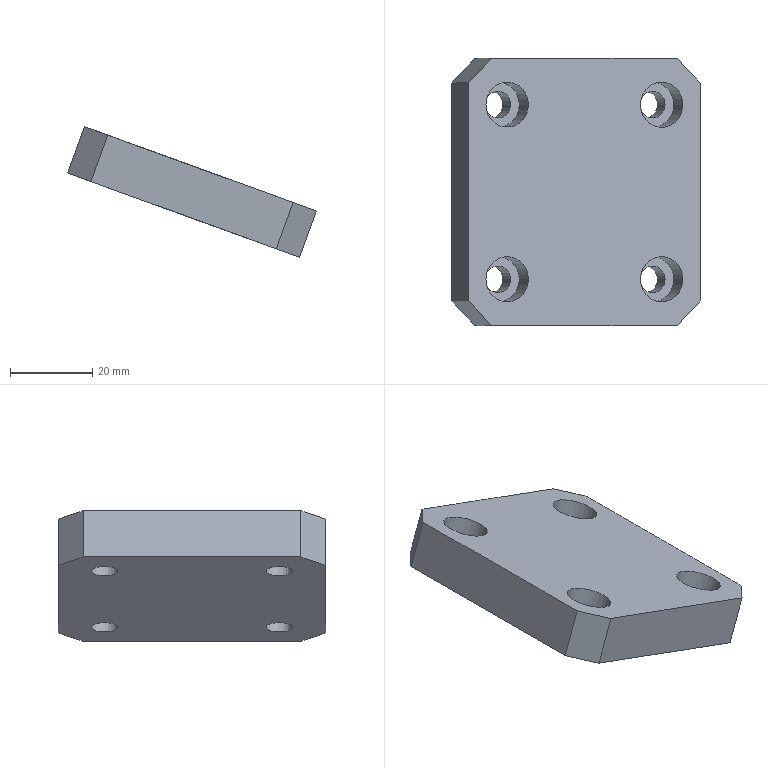Part | STEP file | P011002S002-008 | 1 solid | 22 faces | box 60.486 x 65 x 31.798 mm | volume 42735 mm3 | plane 14 | cylinder 8 | commonest cylinder face diameters 6.5 x4 11 x4